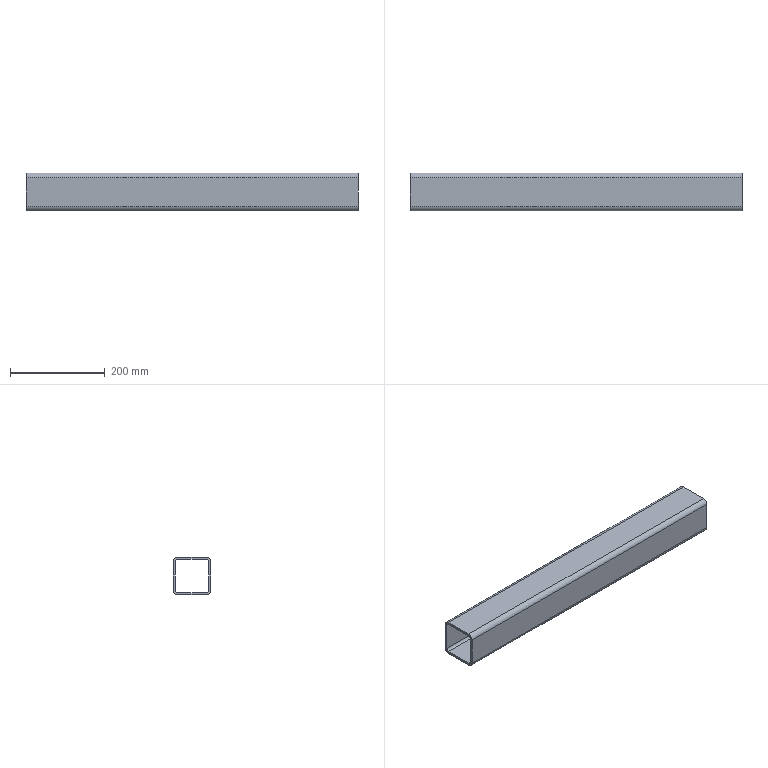Part | SolidWorks | features BaseBody 1 | 1 solid | 18 faces | box 700 x 80 x 80 mm | volume 1004934 mm3 | plane 10 | cylinder 8 | commonest cylinder face diameters 10 x4 20 x4
STEP:
#1=CARTESIAN_POINT('',(-350.,30.,-40.));
#2=VERTEX_POINT('',#1);
#3=CARTESIAN_POINT('',(-350.,40.,-30.));
#4=VERTEX_POINT('',#3);
#5=CARTESIAN_POINT('',(-350.,30.,-30.));
#6=DIRECTION('',(1.,0.,0.));
#7=DIRECTION('',(0.,0.,-1.));
#8=AXIS2_PLACEMENT_3D('',#5,#6,#7);
#9=CIRCLE('',#8,10.);
#10=EDGE_CURVE('',#2,#4,#9,.T.);
#11=ORIENTED_EDGE('',*,*,#10,.T.);
#12=CARTESIAN_POINT('',(350.,40.,-30.));
#13=VERTEX_POINT('',#12);
#14=CARTESIAN_POINT('',(350.,40.,-30.));
#15=DIRECTION('',(-1.,0.,0.));
#16=VECTOR('',#15,1000.);
#17=LINE('',#14,#16);
#18=EDGE_CURVE('',#13,#4,#17,.T.);
#19=ORIENTED_EDGE('',*,*,#18,.F.);
#20=CARTESIAN_POINT('',(350.,30.,-40.));
#21=VERTEX_POINT('',#20);
#22=CARTESIAN_POINT('',(350.,30.,-30.));
#23=DIRECTION('',(1.,0.,0.));
#24=DIRECTION('',(0.,0.,-1.));
#25=AXIS2_PLACEMENT_3D('',#22,#23,#24);
#26=CIRCLE('',#25,10.);
#27=EDGE_CURVE('',#21,#13,#26,.T.);
#28=ORIENTED_EDGE('',*,*,#27,.F.);
#29=CARTESIAN_POINT('',(350.,30.,-40.));
#30=DIRECTION('',(-1.,0.,0.));
#31=VECTOR('',#30,1000.);
#32=LINE('',#29,#31);
#33=EDGE_CURVE('',#21,#2,#32,.T.);
#34=ORIENTED_EDGE('',*,*,#33,.T.);
#35=EDGE_LOOP('',(#11,#19,#28,#34));
#36=FACE_OUTER_BOUND('',#35,.T.);
#37=CARTESIAN_POINT('',(350.,30.,-30.));
#38=DIRECTION('',(-1.,0.,0.));
#39=DIRECTION('',(0.,0.,1.));
#40=AXIS2_PLACEMENT_3D('',#37,#38,#39);
#41=CYLINDRICAL_SURFACE('',#40,10.);
#42=ADVANCED_FACE('',(#36),#41,.T.);
#43=CARTESIAN_POINT('',(-350.,40.,30.));
#44=VERTEX_POINT('',#43);
#45=CARTESIAN_POINT('',(-350.,40.,-30.));
#46=DIRECTION('',(0.,0.,1.));
#47=VECTOR('',#46,1000.);
#48=LINE('',#45,#47);
#49=EDGE_CURVE('',#4,#44,#48,.T.);
#50=ORIENTED_EDGE('',*,*,#49,.T.);
#51=CARTESIAN_POINT('',(350.,40.,30.));
#52=VERTEX_POINT('',#51);
#53=CARTESIAN_POINT('',(350.,40.,30.));
#54=DIRECTION('',(-1.,0.,0.));
#55=VECTOR('',#54,1000.);
#56=LINE('',#53,#55);
#57=EDGE_CURVE('',#52,#44,#56,.T.);
#58=ORIENTED_EDGE('',*,*,#57,.F.);
#59=CARTESIAN_POINT('',(350.,40.,-30.));
#60=DIRECTION('',(0.,0.,1.));
#61=VECTOR('',#60,1000.);
#62=LINE('',#59,#61);
#63=EDGE_CURVE('',#13,#52,#62,.T.);
#64=ORIENTED_EDGE('',*,*,#63,.F.);
#65=ORIENTED_EDGE('',*,*,#18,.T.);
#66=EDGE_LOOP('',(#50,#58,#64,#65));
#67=FACE_OUTER_BOUND('',#66,.T.);
#68=CARTESIAN_POINT('',(350.,40.,-30.));
#69=DIRECTION('',(0.,-1.,0.));
#70=DIRECTION('',(0.,0.,-1.));
#71=AXIS2_PLACEMENT_3D('',#68,#69,#70);
#72=PLANE('',#71);
#73=ADVANCED_FACE('',(#67),#72,.F.);
#74=CARTESIAN_POINT('',(-350.,30.,40.));
#75=VERTEX_POINT('',#74);
#76=CARTESIAN_POINT('',(-350.,30.,30.));
#77=DIRECTION('',(1.,0.,0.));
#78=DIRECTION('',(0.,0.,-1.));
#79=AXIS2_PLACEMENT_3D('',#76,#77,#78);
#80=CIRCLE('',#79,10.);
#81=EDGE_CURVE('',#44,#75,#80,.T.);
#82=ORIENTED_EDGE('',*,*,#81,.T.);
#83=CARTESIAN_POINT('',(350.,30.,40.));
#84=VERTEX_POINT('',#83);
#85=CARTESIAN_POINT('',(350.,30.,40.));
#86=DIRECTION('',(-1.,0.,0.));
#87=VECTOR('',#86,1000.);
#88=LINE('',#85,#87);
#89=EDGE_CURVE('',#84,#75,#88,.T.);
#90=ORIENTED_EDGE('',*,*,#89,.F.);
#91=CARTESIAN_POINT('',(350.,30.,30.));
#92=DIRECTION('',(1.,0.,0.));
#93=DIRECTION('',(0.,0.,-1.));
#94=AXIS2_PLACEMENT_3D('',#91,#92,#93);
#95=CIRCLE('',#94,10.);
#96=EDGE_CURVE('',#52,#84,#95,.T.);
#97=ORIENTED_EDGE('',*,*,#96,.F.);
#98=ORIENTED_EDGE('',*,*,#57,.T.);
#99=EDGE_LOOP('',(#82,#90,#97,#98));
#100=FACE_OUTER_BOUND('',#99,.T.);
#101=CARTESIAN_POINT('',(350.,30.,30.));
#102=DIRECTION('',(-1.,0.,0.));
#103=DIRECTION('',(0.,0.,1.));
#104=AXIS2_PLACEMENT_3D('',#101,#102,#103);
#105=CYLINDRICAL_SURFACE('',#104,10.);
#106=ADVANCED_FACE('',(#100),#105,.T.);
#107=CARTESIAN_POINT('',(-350.,-30.,40.));
#108=VERTEX_POINT('',#107);
#109=CARTESIAN_POINT('',(-350.,-30.,40.));
#110=DIRECTION('',(0.,-1.,0.));
#111=VECTOR('',#110,1000.);
#112=LINE('',#109,#111);
#113=EDGE_CURVE('',#75,#108,#112,.T.);
#114=ORIENTED_EDGE('',*,*,#113,.T.);
#115=CARTESIAN_POINT('',(350.,-30.,40.));
#116=VERTEX_POINT('',#115);
#117=CARTESIAN_POINT('',(350.,-30.,40.));
#118=DIRECTION('',(-1.,0.,0.));
#119=VECTOR('',#118,1000.);
#120=LINE('',#117,#119);
#121=EDGE_CURVE('',#116,#108,#120,.T.);
#122=ORIENTED_EDGE('',*,*,#121,.F.);
#123=CARTESIAN_POINT('',(350.,-30.,40.));
#124=DIRECTION('',(0.,-1.,0.));
#125=VECTOR('',#124,1000.);
#126=LINE('',#123,#125);
#127=EDGE_CURVE('',#84,#116,#126,.T.);
#128=ORIENTED_EDGE('',*,*,#127,.F.);
#129=ORIENTED_EDGE('',*,*,#89,.T.);
#130=EDGE_LOOP('',(#114,#122,#128,#129));
#131=FACE_OUTER_BOUND('',#130,.T.);
#132=CARTESIAN_POINT('',(350.,-30.,40.));
#133=DIRECTION('',(0.,0.,-1.));
#134=DIRECTION('',(-1.,0.,0.));
#135=AXIS2_PLACEMENT_3D('',#132,#133,#134);
#136=PLANE('',#135);
#137=ADVANCED_FACE('',(#131),#136,.F.);
#138=CARTESIAN_POINT('',(-350.,-40.,30.));
#139=VERTEX_POINT('',#138);
#140=CARTESIAN_POINT('',(-350.,-30.,30.));
#141=DIRECTION('',(1.,0.,0.));
#142=DIRECTION('',(0.,0.,-1.));
#143=AXIS2_PLACEMENT_3D('',#140,#141,#142);
#144=CIRCLE('',#143,10.);
#145=EDGE_CURVE('',#108,#139,#144,.T.);
#146=ORIENTED_EDGE('',*,*,#145,.T.);
#147=CARTESIAN_POINT('',(350.,-40.,30.));
#148=VERTEX_POINT('',#147);
#149=CARTESIAN_POINT('',(350.,-40.,30.));
#150=DIRECTION('',(-1.,0.,0.));
#151=VECTOR('',#150,1000.);
#152=LINE('',#149,#151);
#153=EDGE_CURVE('',#148,#139,#152,.T.);
#154=ORIENTED_EDGE('',*,*,#153,.F.);
#155=CARTESIAN_POINT('',(350.,-30.,30.));
#156=DIRECTION('',(1.,0.,0.));
#157=DIRECTION('',(0.,0.,-1.));
#158=AXIS2_PLACEMENT_3D('',#155,#156,#157);
#159=CIRCLE('',#158,10.);
#160=EDGE_CURVE('',#116,#148,#159,.T.);
#161=ORIENTED_EDGE('',*,*,#160,.F.);
#162=ORIENTED_EDGE('',*,*,#121,.T.);
#163=EDGE_LOOP('',(#146,#154,#161,#162));
#164=FACE_OUTER_BOUND('',#163,.T.);
#165=CARTESIAN_POINT('',(350.,-30.,30.));
#166=DIRECTION('',(-1.,0.,0.));
#167=DIRECTION('',(0.,0.,1.));
#168=AXIS2_PLACEMENT_3D('',#165,#166,#167);
#169=CYLINDRICAL_SURFACE('',#168,10.);
#170=ADVANCED_FACE('',(#164),#169,.T.);
#171=CARTESIAN_POINT('',(-350.,-40.,-30.));
#172=VERTEX_POINT('',#171);
#173=CARTESIAN_POINT('',(-350.,-40.,30.));
#174=DIRECTION('',(0.,0.,-1.));
#175=VECTOR('',#174,1000.);
#176=LINE('',#173,#175);
#177=EDGE_CURVE('',#139,#172,#176,.T.);
#178=ORIENTED_EDGE('',*,*,#177,.T.);
#179=CARTESIAN_POINT('',(350.,-40.,-30.));
#180=VERTEX_POINT('',#179);
#181=CARTESIAN_POINT('',(350.,-40.,-30.));
#182=DIRECTION('',(-1.,0.,0.));
#183=VECTOR('',#182,1000.);
#184=LINE('',#181,#183);
#185=EDGE_CURVE('',#180,#172,#184,.T.);
#186=ORIENTED_EDGE('',*,*,#185,.F.);
#187=CARTESIAN_POINT('',(350.,-40.,30.));
#188=DIRECTION('',(0.,0.,-1.));
#189=VECTOR('',#188,1000.);
#190=LINE('',#187,#189);
#191=EDGE_CURVE('',#148,#180,#190,.T.);
#192=ORIENTED_EDGE('',*,*,#191,.F.);
#193=ORIENTED_EDGE('',*,*,#153,.T.);
#194=EDGE_LOOP('',(#178,#186,#192,#193));
#195=FACE_OUTER_BOUND('',#194,.T.);
#196=CARTESIAN_POINT('',(350.,-40.,30.));
#197=DIRECTION('',(0.,1.,0.));
#198=DIRECTION('',(0.,0.,1.));
#199=AXIS2_PLACEMENT_3D('',#196,#197,#198);
#200=PLANE('',#199);
#201=ADVANCED_FACE('',(#195),#200,.F.);
#202=CARTESIAN_POINT('',(-350.,-30.,-40.));
#203=VERTEX_POINT('',#202);
#204=CARTESIAN_POINT('',(-350.,-30.,-30.));
#205=DIRECTION('',(1.,0.,0.));
#206=DIRECTION('',(0.,0.,-1.));
#207=AXIS2_PLACEMENT_3D('',#204,#205,#206);
#208=CIRCLE('',#207,10.);
#209=EDGE_CURVE('',#172,#203,#208,.T.);
#210=ORIENTED_EDGE('',*,*,#209,.T.);
#211=CARTESIAN_POINT('',(350.,-30.,-40.));
#212=VERTEX_POINT('',#211);
#213=CARTESIAN_POINT('',(350.,-30.,-40.));
#214=DIRECTION('',(-1.,0.,0.));
#215=VECTOR('',#214,1000.);
#216=LINE('',#213,#215);
#217=EDGE_CURVE('',#212,#203,#216,.T.);
#218=ORIENTED_EDGE('',*,*,#217,.F.);
#219=CARTESIAN_POINT('',(350.,-30.,-30.));
#220=DIRECTION('',(1.,0.,0.));
#221=DIRECTION('',(0.,0.,-1.));
#222=AXIS2_PLACEMENT_3D('',#219,#220,#221);
#223=CIRCLE('',#222,10.);
#224=EDGE_CURVE('',#180,#212,#223,.T.);
#225=ORIENTED_EDGE('',*,*,#224,.F.);
#226=ORIENTED_EDGE('',*,*,#185,.T.);
#227=EDGE_LOOP('',(#210,#218,#225,#226));
#228=FACE_OUTER_BOUND('',#227,.T.);
#229=CARTESIAN_POINT('',(350.,-30.,-30.));
#230=DIRECTION('',(-1.,0.,0.));
#231=DIRECTION('',(0.,0.,1.));
#232=AXIS2_PLACEMENT_3D('',#229,#230,#231);
#233=CYLINDRICAL_SURFACE('',#232,10.);
#234=ADVANCED_FACE('',(#228),#233,.T.);
#235=CARTESIAN_POINT('',(-350.,35.,30.));
#236=VERTEX_POINT('',#235);
#237=CARTESIAN_POINT('',(-350.,30.,35.));
#238=VERTEX_POINT('',#237);
#239=CARTESIAN_POINT('',(-350.,30.,30.));
#240=DIRECTION('',(1.,0.,0.));
#241=DIRECTION('',(0.,0.,-1.));
#242=AXIS2_PLACEMENT_3D('',#239,#240,#241);
#243=CIRCLE('',#242,5.);
#244=EDGE_CURVE('',#236,#238,#243,.T.);
#245=ORIENTED_EDGE('',*,*,#244,.F.);
#246=CARTESIAN_POINT('',(350.,35.,30.));
#247=VERTEX_POINT('',#246);
#248=CARTESIAN_POINT('',(350.,35.,30.));
#249=DIRECTION('',(-1.,0.,0.));
#250=VECTOR('',#249,1000.);
#251=LINE('',#248,#250);
#252=EDGE_CURVE('',#247,#236,#251,.T.);
#253=ORIENTED_EDGE('',*,*,#252,.F.);
#254=CARTESIAN_POINT('',(350.,30.,35.));
#255=VERTEX_POINT('',#254);
#256=CARTESIAN_POINT('',(350.,30.,30.));
#257=DIRECTION('',(1.,0.,0.));
#258=DIRECTION('',(0.,0.,-1.));
#259=AXIS2_PLACEMENT_3D('',#256,#257,#258);
#260=CIRCLE('',#259,5.);
#261=EDGE_CURVE('',#247,#255,#260,.T.);
#262=ORIENTED_EDGE('',*,*,#261,.T.);
#263=CARTESIAN_POINT('',(350.,30.,35.));
#264=DIRECTION('',(-1.,0.,0.));
#265=VECTOR('',#264,1000.);
#266=LINE('',#263,#265);
#267=EDGE_CURVE('',#255,#238,#266,.T.);
#268=ORIENTED_EDGE('',*,*,#267,.T.);
#269=EDGE_LOOP('',(#245,#253,#262,#268));
#270=FACE_OUTER_BOUND('',#269,.T.);
#271=CARTESIAN_POINT('',(350.,30.,30.));
#272=DIRECTION('',(-1.,0.,0.));
#273=DIRECTION('',(0.,0.,1.));
#274=AXIS2_PLACEMENT_3D('',#271,#272,#273);
#275=CYLINDRICAL_SURFACE('',#274,5.);
#276=ADVANCED_FACE('',(#270),#275,.F.);
#277=CARTESIAN_POINT('',(-350.,35.,-30.));
#278=VERTEX_POINT('',#277);
#279=CARTESIAN_POINT('',(-350.,35.,-30.));
#280=DIRECTION('',(0.,0.,1.));
#281=VECTOR('',#280,1000.);
#282=LINE('',#279,#281);
#283=EDGE_CURVE('',#278,#236,#282,.T.);
#284=ORIENTED_EDGE('',*,*,#283,.F.);
#285=CARTESIAN_POINT('',(350.,35.,-30.));
#286=VERTEX_POINT('',#285);
#287=CARTESIAN_POINT('',(350.,35.,-30.));
#288=DIRECTION('',(-1.,0.,0.));
#289=VECTOR('',#288,1000.);
#290=LINE('',#287,#289);
#291=EDGE_CURVE('',#286,#278,#290,.T.);
#292=ORIENTED_EDGE('',*,*,#291,.F.);
#293=CARTESIAN_POINT('',(350.,35.,-30.));
#294=DIRECTION('',(0.,0.,1.));
#295=VECTOR('',#294,1000.);
#296=LINE('',#293,#295);
#297=EDGE_CURVE('',#286,#247,#296,.T.);
#298=ORIENTED_EDGE('',*,*,#297,.T.);
#299=ORIENTED_EDGE('',*,*,#252,.T.);
#300=EDGE_LOOP('',(#284,#292,#298,#299));
#301=FACE_OUTER_BOUND('',#300,.T.);
#302=CARTESIAN_POINT('',(350.,35.,-30.));
#303=DIRECTION('',(0.,-1.,0.));
#304=DIRECTION('',(0.,0.,-1.));
#305=AXIS2_PLACEMENT_3D('',#302,#303,#304);
#306=PLANE('',#305);
#307=ADVANCED_FACE('',(#301),#306,.T.);
#308=CARTESIAN_POINT('',(-350.,30.,-35.));
#309=VERTEX_POINT('',#308);
#310=CARTESIAN_POINT('',(-350.,30.,-30.));
#311=DIRECTION('',(1.,0.,0.));
#312=DIRECTION('',(0.,0.,-1.));
#313=AXIS2_PLACEMENT_3D('',#310,#311,#312);
#314=CIRCLE('',#313,5.);
#315=EDGE_CURVE('',#309,#278,#314,.T.);
#316=ORIENTED_EDGE('',*,*,#315,.F.);
#317=CARTESIAN_POINT('',(350.,30.,-35.));
#318=VERTEX_POINT('',#317);
#319=CARTESIAN_POINT('',(350.,30.,-35.));
#320=DIRECTION('',(-1.,0.,0.));
#321=VECTOR('',#320,1000.);
#322=LINE('',#319,#321);
#323=EDGE_CURVE('',#318,#309,#322,.T.);
#324=ORIENTED_EDGE('',*,*,#323,.F.);
#325=CARTESIAN_POINT('',(350.,30.,-30.));
#326=DIRECTION('',(1.,0.,0.));
#327=DIRECTION('',(0.,0.,-1.));
#328=AXIS2_PLACEMENT_3D('',#325,#326,#327);
#329=CIRCLE('',#328,5.);
#330=EDGE_CURVE('',#318,#286,#329,.T.);
#331=ORIENTED_EDGE('',*,*,#330,.T.);
#332=ORIENTED_EDGE('',*,*,#291,.T.);
#333=EDGE_LOOP('',(#316,#324,#331,#332));
#334=FACE_OUTER_BOUND('',#333,.T.);
#335=CARTESIAN_POINT('',(350.,30.,-30.));
#336=DIRECTION('',(-1.,0.,0.));
#337=DIRECTION('',(0.,0.,1.));
#338=AXIS2_PLACEMENT_3D('',#335,#336,#337);
#339=CYLINDRICAL_SURFACE('',#338,5.);
#340=ADVANCED_FACE('',(#334),#339,.F.);
#341=CARTESIAN_POINT('',(-350.,-30.,-35.));
#342=VERTEX_POINT('',#341);
#343=CARTESIAN_POINT('',(-350.,30.,-35.));
#344=DIRECTION('',(0.,1.,0.));
#345=VECTOR('',#344,1000.);
#346=LINE('',#343,#345);
#347=EDGE_CURVE('',#342,#309,#346,.T.);
#348=ORIENTED_EDGE('',*,*,#347,.F.);
#349=CARTESIAN_POINT('',(350.,-30.,-35.));
#350=VERTEX_POINT('',#349);
#351=CARTESIAN_POINT('',(350.,-30.,-35.));
#352=DIRECTION('',(-1.,0.,0.));
#353=VECTOR('',#352,1000.);
#354=LINE('',#351,#353);
#355=EDGE_CURVE('',#350,#342,#354,.T.);
#356=ORIENTED_EDGE('',*,*,#355,.F.);
#357=CARTESIAN_POINT('',(350.,30.,-35.));
#358=DIRECTION('',(0.,1.,0.));
#359=VECTOR('',#358,1000.);
#360=LINE('',#357,#359);
#361=EDGE_CURVE('',#350,#318,#360,.T.);
#362=ORIENTED_EDGE('',*,*,#361,.T.);
#363=ORIENTED_EDGE('',*,*,#323,.T.);
#364=EDGE_LOOP('',(#348,#356,#362,#363));
#365=FACE_OUTER_BOUND('',#364,.T.);
#366=CARTESIAN_POINT('',(350.,30.,-35.));
#367=DIRECTION('',(0.,0.,1.));
#368=DIRECTION('',(1.,0.,0.));
#369=AXIS2_PLACEMENT_3D('',#366,#367,#368);
#370=PLANE('',#369);
#371=ADVANCED_FACE('',(#365),#370,.T.);
#372=CARTESIAN_POINT('',(-350.,-35.,-30.));
#373=VERTEX_POINT('',#372);
#374=CARTESIAN_POINT('',(-350.,-30.,-30.));
#375=DIRECTION('',(1.,0.,0.));
#376=DIRECTION('',(0.,0.,-1.));
#377=AXIS2_PLACEMENT_3D('',#374,#375,#376);
#378=CIRCLE('',#377,5.);
#379=EDGE_CURVE('',#373,#342,#378,.T.);
#380=ORIENTED_EDGE('',*,*,#379,.F.);
#381=CARTESIAN_POINT('',(350.,-35.,-30.));
#382=VERTEX_POINT('',#381);
#383=CARTESIAN_POINT('',(350.,-35.,-30.));
#384=DIRECTION('',(-1.,0.,0.));
#385=VECTOR('',#384,1000.);
#386=LINE('',#383,#385);
#387=EDGE_CURVE('',#382,#373,#386,.T.);
#388=ORIENTED_EDGE('',*,*,#387,.F.);
#389=CARTESIAN_POINT('',(350.,-30.,-30.));
#390=DIRECTION('',(1.,0.,0.));
#391=DIRECTION('',(0.,0.,-1.));
#392=AXIS2_PLACEMENT_3D('',#389,#390,#391);
#393=CIRCLE('',#392,5.);
#394=EDGE_CURVE('',#382,#350,#393,.T.);
#395=ORIENTED_EDGE('',*,*,#394,.T.);
#396=ORIENTED_EDGE('',*,*,#355,.T.);
#397=EDGE_LOOP('',(#380,#388,#395,#396));
#398=FACE_OUTER_BOUND('',#397,.T.);
#399=CARTESIAN_POINT('',(350.,-30.,-30.));
#400=DIRECTION('',(-1.,0.,0.));
#401=DIRECTION('',(0.,0.,1.));
#402=AXIS2_PLACEMENT_3D('',#399,#400,#401);
#403=CYLINDRICAL_SURFACE('',#402,5.);
#404=ADVANCED_FACE('',(#398),#403,.F.);
#405=CARTESIAN_POINT('',(-350.,-35.,30.));
#406=VERTEX_POINT('',#405);
#407=CARTESIAN_POINT('',(-350.,-35.,30.));
#408=DIRECTION('',(0.,0.,-1.));
#409=VECTOR('',#408,1000.);
#410=LINE('',#407,#409);
#411=EDGE_CURVE('',#406,#373,#410,.T.);
#412=ORIENTED_EDGE('',*,*,#411,.F.);
#413=CARTESIAN_POINT('',(350.,-35.,30.));
#414=VERTEX_POINT('',#413);
#415=CARTESIAN_POINT('',(350.,-35.,30.));
#416=DIRECTION('',(-1.,0.,0.));
#417=VECTOR('',#416,1000.);
#418=LINE('',#415,#417);
#419=EDGE_CURVE('',#414,#406,#418,.T.);
#420=ORIENTED_EDGE('',*,*,#419,.F.);
#421=CARTESIAN_POINT('',(350.,-35.,30.));
#422=DIRECTION('',(0.,0.,-1.));
#423=VECTOR('',#422,1000.);
#424=LINE('',#421,#423);
#425=EDGE_CURVE('',#414,#382,#424,.T.);
#426=ORIENTED_EDGE('',*,*,#425,.T.);
#427=ORIENTED_EDGE('',*,*,#387,.T.);
#428=EDGE_LOOP('',(#412,#420,#426,#427));
#429=FACE_OUTER_BOUND('',#428,.T.);
#430=CARTESIAN_POINT('',(350.,-35.,30.));
#431=DIRECTION('',(0.,1.,0.));
#432=DIRECTION('',(0.,0.,1.));
#433=AXIS2_PLACEMENT_3D('',#430,#431,#432);
#434=PLANE('',#433);
#435=ADVANCED_FACE('',(#429),#434,.T.);
#436=CARTESIAN_POINT('',(-350.,-30.,35.));
#437=VERTEX_POINT('',#436);
#438=CARTESIAN_POINT('',(-350.,-30.,30.));
#439=DIRECTION('',(1.,0.,0.));
#440=DIRECTION('',(0.,0.,-1.));
#441=AXIS2_PLACEMENT_3D('',#438,#439,#440);
#442=CIRCLE('',#441,5.);
#443=EDGE_CURVE('',#437,#406,#442,.T.);
#444=ORIENTED_EDGE('',*,*,#443,.F.);
#445=CARTESIAN_POINT('',(350.,-30.,35.));
#446=VERTEX_POINT('',#445);
#447=CARTESIAN_POINT('',(350.,-30.,35.));
#448=DIRECTION('',(-1.,0.,0.));
#449=VECTOR('',#448,1000.);
#450=LINE('',#447,#449);
#451=EDGE_CURVE('',#446,#437,#450,.T.);
#452=ORIENTED_EDGE('',*,*,#451,.F.);
#453=CARTESIAN_POINT('',(350.,-30.,30.));
#454=DIRECTION('',(1.,0.,0.));
#455=DIRECTION('',(0.,0.,-1.));
#456=AXIS2_PLACEMENT_3D('',#453,#454,#455);
#457=CIRCLE('',#456,5.);
#458=EDGE_CURVE('',#446,#414,#457,.T.);
#459=ORIENTED_EDGE('',*,*,#458,.T.);
#460=ORIENTED_EDGE('',*,*,#419,.T.);
#461=EDGE_LOOP('',(#444,#452,#459,#460));
#462=FACE_OUTER_BOUND('',#461,.T.);
#463=CARTESIAN_POINT('',(350.,-30.,30.));
#464=DIRECTION('',(-1.,0.,0.));
#465=DIRECTION('',(0.,0.,1.));
#466=AXIS2_PLACEMENT_3D('',#463,#464,#465);
#467=CYLINDRICAL_SURFACE('',#466,5.);
#468=ADVANCED_FACE('',(#462),#467,.F.);
#469=CARTESIAN_POINT('',(-350.,-30.,35.));
#470=DIRECTION('',(0.,-1.,0.));
#471=VECTOR('',#470,1000.);
#472=LINE('',#469,#471);
#473=EDGE_CURVE('',#238,#437,#472,.T.);
#474=ORIENTED_EDGE('',*,*,#473,.F.);
#475=ORIENTED_EDGE('',*,*,#267,.F.);
#476=CARTESIAN_POINT('',(350.,-30.,35.));
#477=DIRECTION('',(0.,-1.,0.));
#478=VECTOR('',#477,1000.);
#479=LINE('',#476,#478);
#480=EDGE_CURVE('',#255,#446,#479,.T.);
#481=ORIENTED_EDGE('',*,*,#480,.T.);
#482=ORIENTED_EDGE('',*,*,#451,.T.);
#483=EDGE_LOOP('',(#474,#475,#481,#482));
#484=FACE_OUTER_BOUND('',#483,.T.);
#485=CARTESIAN_POINT('',(350.,-30.,35.));
#486=DIRECTION('',(0.,0.,-1.));
#487=DIRECTION('',(-1.,0.,0.));
#488=AXIS2_PLACEMENT_3D('',#485,#486,#487);
#489=PLANE('',#488);
#490=ADVANCED_FACE('',(#484),#489,.T.);
#491=CARTESIAN_POINT('',(-350.,30.,-40.));
#492=DIRECTION('',(0.,1.,0.));
#493=VECTOR('',#492,1000.);
#494=LINE('',#491,#493);
#495=EDGE_CURVE('',#203,#2,#494,.T.);
#496=ORIENTED_EDGE('',*,*,#495,.T.);
#497=ORIENTED_EDGE('',*,*,#33,.F.);
#498=CARTESIAN_POINT('',(350.,30.,-40.));
#499=DIRECTION('',(0.,1.,0.));
#500=VECTOR('',#499,1000.);
#501=LINE('',#498,#500);
#502=EDGE_CURVE('',#212,#21,#501,.T.);
#503=ORIENTED_EDGE('',*,*,#502,.F.);
#504=ORIENTED_EDGE('',*,*,#217,.T.);
#505=EDGE_LOOP('',(#496,#497,#503,#504));
#506=FACE_OUTER_BOUND('',#505,.T.);
#507=CARTESIAN_POINT('',(350.,30.,-40.));
#508=DIRECTION('',(0.,0.,1.));
#509=DIRECTION('',(1.,0.,0.));
#510=AXIS2_PLACEMENT_3D('',#507,#508,#509);
#511=PLANE('',#510);
#512=ADVANCED_FACE('',(#506),#511,.F.);
#513=ORIENTED_EDGE('',*,*,#261,.F.);
#514=ORIENTED_EDGE('',*,*,#297,.F.);
#515=ORIENTED_EDGE('',*,*,#330,.F.);
#516=ORIENTED_EDGE('',*,*,#361,.F.);
#517=ORIENTED_EDGE('',*,*,#394,.F.);
#518=ORIENTED_EDGE('',*,*,#425,.F.);
#519=ORIENTED_EDGE('',*,*,#458,.F.);
#520=ORIENTED_EDGE('',*,*,#480,.F.);
#521=EDGE_LOOP('',(#513,#514,#515,#516,#517,#518,#519,#520));
#522=FACE_BOUND('',#521,.T.);
#523=ORIENTED_EDGE('',*,*,#27,.T.);
#524=ORIENTED_EDGE('',*,*,#63,.T.);
#525=ORIENTED_EDGE('',*,*,#96,.T.);
#526=ORIENTED_EDGE('',*,*,#127,.T.);
#527=ORIENTED_EDGE('',*,*,#160,.T.);
#528=ORIENTED_EDGE('',*,*,#191,.T.);
#529=ORIENTED_EDGE('',*,*,#224,.T.);
#530=ORIENTED_EDGE('',*,*,#502,.T.);
#531=EDGE_LOOP('',(#523,#524,#525,#526,#527,#528,#529,#530));
#532=FACE_OUTER_BOUND('',#531,.T.);
#533=CARTESIAN_POINT('',(350.,30.,-30.));
#534=DIRECTION('',(1.,0.,0.));
#535=DIRECTION('',(0.,0.,-1.));
#536=AXIS2_PLACEMENT_3D('',#533,#534,#535);
#537=PLANE('',#536);
#538=ADVANCED_FACE('',(#522,#532),#537,.T.);
#539=ORIENTED_EDGE('',*,*,#244,.T.);
#540=ORIENTED_EDGE('',*,*,#473,.T.);
#541=ORIENTED_EDGE('',*,*,#443,.T.);
#542=ORIENTED_EDGE('',*,*,#411,.T.);
#543=ORIENTED_EDGE('',*,*,#379,.T.);
#544=ORIENTED_EDGE('',*,*,#347,.T.);
#545=ORIENTED_EDGE('',*,*,#315,.T.);
#546=ORIENTED_EDGE('',*,*,#283,.T.);
#547=EDGE_LOOP('',(#539,#540,#541,#542,#543,#544,#545,#546));
#548=FACE_BOUND('',#547,.T.);
#549=ORIENTED_EDGE('',*,*,#10,.F.);
#550=ORIENTED_EDGE('',*,*,#495,.F.);
#551=ORIENTED_EDGE('',*,*,#209,.F.);
#552=ORIENTED_EDGE('',*,*,#177,.F.);
#553=ORIENTED_EDGE('',*,*,#145,.F.);
#554=ORIENTED_EDGE('',*,*,#113,.F.);
#555=ORIENTED_EDGE('',*,*,#81,.F.);
#556=ORIENTED_EDGE('',*,*,#49,.F.);
#557=EDGE_LOOP('',(#549,#550,#551,#552,#553,#554,#555,#556));
#558=FACE_OUTER_BOUND('',#557,.T.);
#559=CARTESIAN_POINT('',(-350.,30.,-30.));
#560=DIRECTION('',(1.,0.,0.));
#561=DIRECTION('',(0.,0.,-1.));
#562=AXIS2_PLACEMENT_3D('',#559,#560,#561);
#563=PLANE('',#562);
#564=ADVANCED_FACE('',(#548,#558),#563,.F.);
#565=CLOSED_SHELL('',(#42,#73,#106,#137,#170,#201,#234,#276,#307,#340,#371,#404,#435,#468,#490,#512,#538,#564));
#566=MANIFOLD_SOLID_BREP('',#565);
#567=CARTESIAN_POINT('',(0.,0.,0.));
#568=DIRECTION('',(0.,0.,1.));
#569=DIRECTION('',(1.,0.,0.));
#570=AXIS2_PLACEMENT_3D('',#567,#568,#569);
#571=(LENGTH_UNIT()NAMED_UNIT(*)SI_UNIT(.MILLI.,.METRE.));
#572=UNCERTAINTY_MEASURE_WITH_UNIT(LENGTH_MEASURE(0.00001),#571,'','');
#573=(NAMED_UNIT(*)PLANE_ANGLE_UNIT()SI_UNIT($,.RADIAN.));
#574=(NAMED_UNIT(*)SI_UNIT($,.STERADIAN.)SOLID_ANGLE_UNIT());
#575=(GEOMETRIC_REPRESENTATION_CONTEXT(3)GLOBAL_UNCERTAINTY_ASSIGNED_CONTEXT((#572))GLOBAL_UNIT_ASSIGNED_CONTEXT((#571,#573,#574))REPRESENTATION_CONTEXT('',''));
#576=ADVANCED_BREP_SHAPE_REPRESENTATION('',(#566,#570),#575);